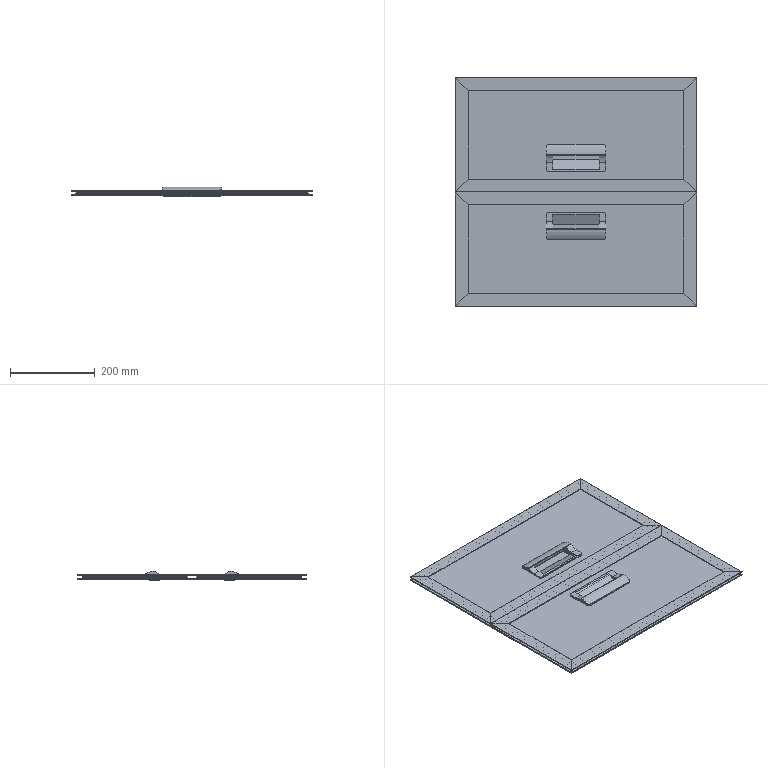Part | SolidWorks | 12 solids | 318 faces | box 570 x 540 x 23.592 mm | volume 1718073 mm3 | plane 206 | cylinder 88 | spline 8 | cone 8 | torus 8 | commonest cylinder face diameters 2 x44 4 x8 8 x8 10 x8 12 x8 52 x6